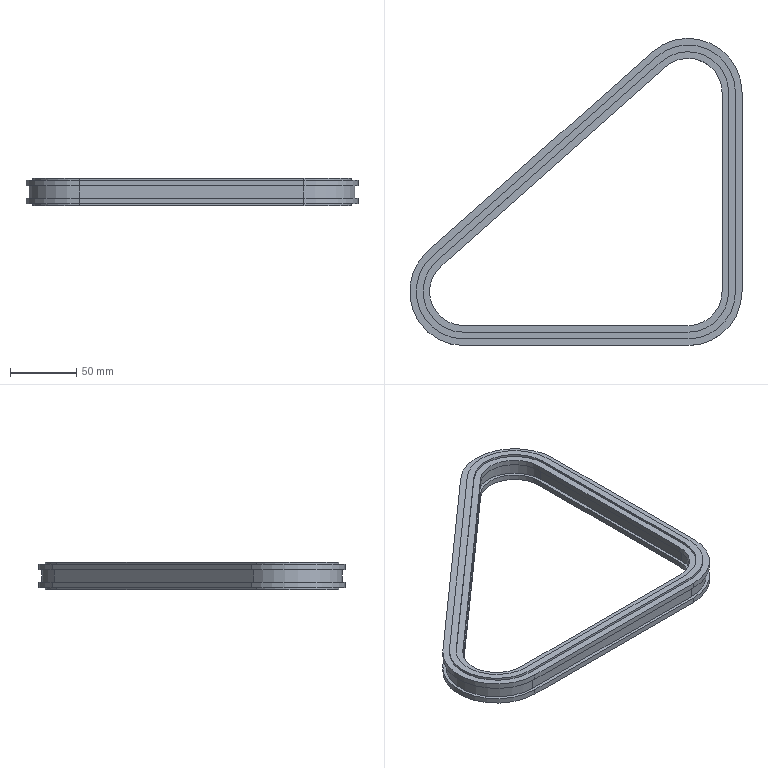Part | STEP file | Roller chain_3 | 1 solid | 70 faces | box 250.346 x 231.346 x 21.082 mm | volume 177949 mm3 | plane 40 | cylinder 30 | commonest cylinder face diameters 51.324 x6 61.255 x6 71.415 x6 81.346 x6 56.175 x3 76.495 x3